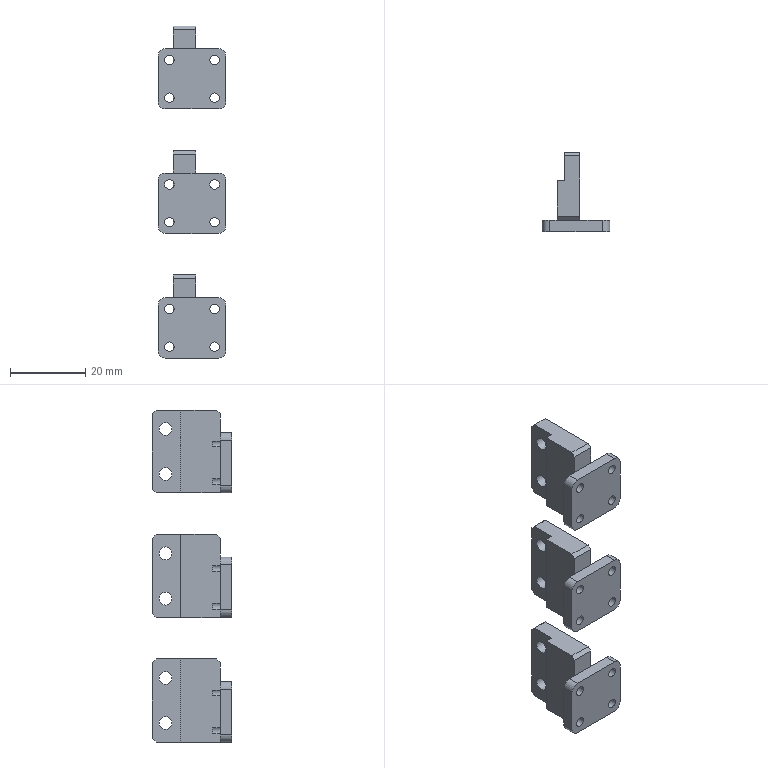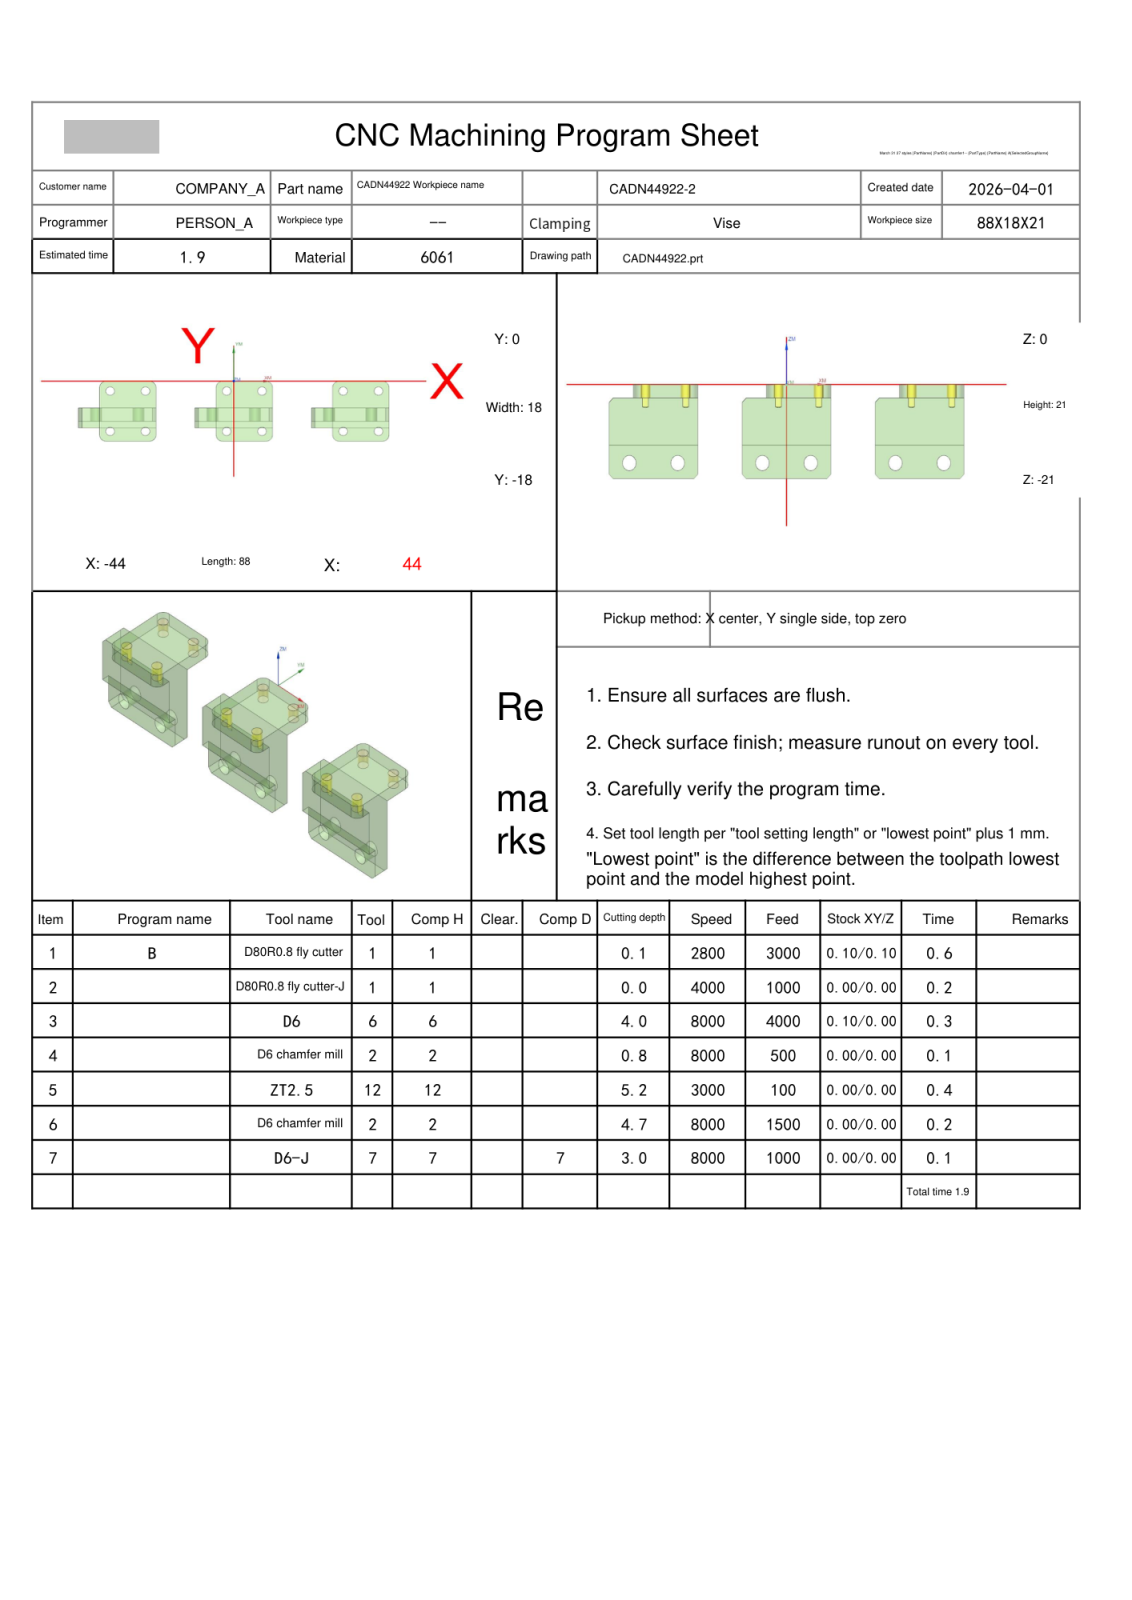NC program | NX | posted by the shop | part box 18 x 21 x 88 mm
Whole program:
%
O0001
(Machine time: 3.18 MIN)
(===Total Tool:5===)
(T1=D80R0.8 fly cutter D=80.  R=0.8  D-  H01 Z=0.    )
(T6=D6      D=6.   R=0.   D-  H06 Z=-4.   )
(T2=D6 chamfer mill   D=6.   R=0.   D-  H02 Z=-4.7  )
(T12=ZT2.5  D=2.5  DR_a=118 D-  H12 Z=-5.15 )
(T7=D6-J    D=6.   R=0.   D7  H07 Z=-3.   )
G80 G90 G17 G49 G40
G91 G28 Z0
M01
N1 T01 M06
(D80R0.8 fly cutter  D=80. R=0.8 H=01 ce=0.10 di=0.10)
G00 G90 G54 X96.097 Y-9. M03 S2800
G43 H01 Z20.
M08
Z5.014
G01 Z3.014 F3000.
X84.097
X-84.097
X-96.097
Z5.014
G00 X96.097
Z4.529
G01 Z2.529
X84.097
X-84.097
X-96.097
Z4.529
G00 X96.097
Z4.043
G01 Z2.043
X84.097
X-84.097
X-96.097
Z4.043
G00 X96.097
Z3.557
G01 Z1.557
X84.097
X-84.097
X-96.097
Z3.557
G00 Z20.
X96.097
Z3.071
G01 Z1.071
X84.097
X-84.097
X-96.097
Z3.071
G00 Z20.
X96.097
Z2.586
G01 Z.586
X84.097
X-84.097
X-96.097
Z2.586
G00 Z20.
X96.097
Z2.1
G01 Z.1
X84.097
X-84.097
X-96.097
Z2.1
G00 Z20.
G91 G28 Z0.0
M05
M09
G91 G28 Z0.0
M01
N2 T01 M06
(D80R0.8 fly cutter-J  D=80. R=0.8 H=01 ce=0.00 di=0.00)
G00 G90 G54 X95.999 Y-9. M03 S4000
G43 H01 Z20.
M08
Z2.
G01 Z0.0 F1000.
X83.999
X-83.999
X-95.999
Z2.
G00 Z20.
G91 G28 Z0.0
M05
M09
G91 G28 Z0.0
M01
N3 T06 M06
(D6  D=6. R=0. H=06 ce=0.10 di=0.10)
G00 G90 G54 X-45.6 Y-2. M03 S8000
G43 H06 Z13.8
M08
Z1.017
G01 Z-.483 F3000.
Y-5.06
Y-16.
G03 X-45.589 Y-16.462 I9.6 J0.0
X-45.097 Y-17.023 I.599 J.029
G01 X-41.71 Y-17.641
X-41.602 Y-17.651
G03 X-41.002 Y-17.051 I0.0 J.6
G01 X-41.013 Y-16.94
G02 X-41.1 Y-16. I5.013 J.94
G01 Y-5.06
Y-2.06
X-44.1 Y-2.
Z1.017
G00 X-45.6
Z.533
G01 Z-.967
Y-5.06
Y-16.
G03 X-45.589 Y-16.462 I9.6 J0.0
X-45.097 Y-17.023 I.599 J.029
G01 X-41.71 Y-17.641
X-41.602 Y-17.651
G03 X-41.002 Y-17.051 I0.0 J.6
G01 X-41.013 Y-16.94
G02 X-41.1 Y-16. I5.013 J.94
G01 Y-5.06
Y-2.06
X-44.1 Y-2.
Z.533
G00 X-45.6
Z.05
G01 Z-1.45
Y-5.06
Y-16.
G03 X-45.589 Y-16.462 I9.6 J0.0
X-45.097 Y-17.023 I.599 J.029
G01 X-41.71 Y-17.641
X-41.602 Y-17.651
G03 X-41.002 Y-17.051 I0.0 J.6
G01 X-41.013 Y-16.94
G02 X-41.1 Y-16. I5.013 J.94
G01 Y-5.06
Y-2.06
X-44.1 Y-2.
Z.05
G00 X-45.6
Z-.433
G01 Z-1.933
Y-5.06
Y-16.
G03 X-45.589 Y-16.462 I9.6 J0.0
X-45.097 Y-17.023 I.599 J.029
G01 X-41.71 Y-17.641
X-41.602 Y-17.651
G03 X-41.002 Y-17.051 I0.0 J.6
G01 X-41.013 Y-16.94
G02 X-41.1 Y-16. I5.013 J.94
G01 Y-5.06
Y-2.06
X-44.1 Y-2.
Z-.433
G00 X-45.6
Z-.917
G01 Z-2.417
Y-5.06
Y-16.
G03 X-45.589 Y-16.462 I9.6 J0.0
X-45.097 Y-17.023 I.599 J.029
G01 X-41.71 Y-17.641
X-41.602 Y-17.651
G03 X-41.002 Y-17.051 I0.0 J.6
G01 X-41.013 Y-16.94
G02 X-41.1 Y-16. I5.013 J.94
G01 Y-5.06
Y-2.06
X-44.1 Y-2.
Z-.917
G00 X-45.6
Z-1.4
G01 Z-2.9
Y-5.06
Y-16.
G03 X-45.589 Y-16.462 I9.6 J0.0
X-45.097 Y-17.023 I.599 J.029
G01 X-41.71 Y-17.641
X-41.602 Y-17.651
G03 X-41.002 Y-17.051 I0.0 J.6
G01 X-41.013 Y-16.94
G02 X-41.1 Y-16. I5.013 J.94
G01 Y-5.06
Y-2.06
X-44.1 Y-2.
Z-1.4
G00 Z13.8
X-12.6
Z1.017
G01 Z-.483
Y-5.06
Y-16.
G03 X-12.589 Y-16.462 I9.6 J0.0
X-12.097 Y-17.023 I.599 J.029
G01 X-8.71 Y-17.641
X-8.602 Y-17.651
G03 X-8.002 Y-17.051 I0.0 J.6
G01 X-8.013 Y-16.94
G02 X-8.1 Y-16. I5.013 J.94
G01 Y-5.06
Y-2.06
X-11.1 Y-2.
Z1.017
G00 X-12.6
Z.533
G01 Z-.967
Y-5.06
Y-16.
G03 X-12.589 Y-16.462 I9.6 J0.0
X-12.097 Y-17.023 I.599 J.029
G01 X-8.71 Y-17.641
X-8.602 Y-17.651
G03 X-8.002 Y-17.051 I0.0 J.6
G01 X-8.013 Y-16.94
G02 X-8.1 Y-16. I5.013 J.94
G01 Y-5.06
Y-2.06
X-11.1 Y-2.
Z.533
G00 X-12.6
Z.05
G01 Z-1.45
Y-5.06
Y-16.
G03 X-12.589 Y-16.462 I9.6 J0.0
X-12.097 Y-17.023 I.599 J.029
G01 X-8.71 Y-17.641
X-8.602 Y-17.651
G03 X-8.002 Y-17.051 I0.0 J.6
G01 X-8.013 Y-16.94
G02 X-8.1 Y-16. I5.013 J.94
G01 Y-5.06
Y-2.06
X-11.1 Y-2.
Z.05
G00 X-12.6
Z-.433
G01 Z-1.933
Y-5.06
Y-16.
G03 X-12.589 Y-16.462 I9.6 J0.0
X-12.097 Y-17.023 I.599 J.029
G01 X-8.71 Y-17.641
X-8.602 Y-17.651
G03 X-8.002 Y-17.051 I0.0 J.6
G01 X-8.013 Y-16.94
G02 X-8.1 Y-16. I5.013 J.94
G01 Y-5.06
Y-2.06
X-11.1 Y-2.
Z-.433
G00 X-12.6
Z-.917
G01 Z-2.417
Y-5.06
Y-16.
G03 X-12.589 Y-16.462 I9.6 J0.0
X-12.097 Y-17.023 I.599 J.029
G01 X-8.71 Y-17.641
X-8.602 Y-17.651
G03 X-8.002 Y-17.051 I0.0 J.6
G01 X-8.013 Y-16.94
G02 X-8.1 Y-16. I5.013 J.94
G01 Y-5.06
Y-2.06
X-11.1 Y-2.
Z-.917
G00 X-12.6
Z-1.4
G01 Z-2.9
Y-5.06
Y-16.
G03 X-12.589 Y-16.462 I9.6 J0.0
X-12.097 Y-17.023 I.599 J.029
G01 X-8.71 Y-17.641
X-8.602 Y-17.651
G03 X-8.002 Y-17.051 I0.0 J.6
G01 X-8.013 Y-16.94
G02 X-8.1 Y-16. I5.013 J.94
G01 Y-5.06
Y-2.06
X-11.1 Y-2.
Z-1.4
G00 Z13.8
X20.4
Z1.017
G01 Z-.483
Y-5.06
Y-16.
G03 X20.411 Y-16.462 I9.6 J0.0
X20.903 Y-17.023 I.599 J.029
G01 X24.29 Y-17.641
X24.398 Y-17.651
G03 X24.998 Y-17.051 I0.0 J.6
G01 X24.987 Y-16.94
G02 X24.9 Y-16. I5.013 J.94
G01 Y-5.06
Y-2.06
X21.9 Y-2.
Z1.017
G00 X20.4
Z.533
G01 Z-.967
Y-5.06
Y-16.
G03 X20.411 Y-16.462 I9.6 J0.0
X20.903 Y-17.023 I.599 J.029
G01 X24.29 Y-17.641
X24.398 Y-17.651
G03 X24.998 Y-17.051 I0.0 J.6
G01 X24.987 Y-16.94
G02 X24.9 Y-16. I5.013 J.94
G01 Y-5.06
Y-2.06
X21.9 Y-2.
Z.533
G00 X20.4
Z.05
G01 Z-1.45
Y-5.06
Y-16.
G03 X20.411 Y-16.462 I9.6 J0.0
X20.903 Y-17.023 I.599 J.029
G01 X24.29 Y-17.641
X24.398 Y-17.651
G03 X24.998 Y-17.051 I0.0 J.6
G01 X24.987 Y-16.94
G02 X24.9 Y-16. I5.013 J.94
G01 Y-5.06
Y-2.06
X21.9 Y-2.
Z.05
G00 X20.4
Z-.433
G01 Z-1.933
Y-5.06
Y-16.
G03 X20.411 Y-16.462 I9.6 J0.0
X20.903 Y-17.023 I.599 J.029
G01 X24.29 Y-17.641
X24.398 Y-17.651
G03 X24.998 Y-17.051 I0.0 J.6
G01 X24.987 Y-16.94
G02 X24.9 Y-16. I5.013 J.94
G01 Y-5.06
Y-2.06
X21.9 Y-2.
Z-.433
G00 X20.4
Z-.917
G01 Z-2.417
Y-5.06
Y-16.
G03 X20.411 Y-16.462 I9.6 J0.0
X20.903 Y-17.023 I.599 J.029
G01 X24.29 Y-17.641
X24.398 Y-17.651
G03 X24.998 Y-17.051 I0.0 J.6
G01 X24.987 Y-16.94
G02 X24.9 Y-16. I5.013 J.94
G01 Y-5.06
Y-2.06
X21.9 Y-2.
Z-.917
G00 X20.4
Z-1.4
G01 Z-2.9
Y-5.06
Y-16.
G03 X20.411 Y-16.462 I9.6 J0.0
X20.903 Y-17.023 I.599 J.029
G01 X24.29 Y-17.641
X24.398 Y-17.651
G03 X24.998 Y-17.051 I0.0 J.6
G01 X24.987 Y-16.94
G02 X24.9 Y-16. I5.013 J.94
G01 Y-5.06
Y-2.06
X21.9 Y-2.
Z-1.4
G00 Z13.8
G00 G90 X-46.185 Y-20.358 M03 S7000
Z13.8
Z-2.641
G01 Z-3.141 F4000.
X-46.239 Y-15.071
X-46.241 Y-14.87
Y-7.13
X-46.239 Y-6.928
X-46.312 Z-3.212
X-46.381 Z-3.283
X-46.383 Y-7.13
Y-14.87
X-46.381 Y-15.071
X-46.454 Z-3.354
X-46.522 Z-3.424
X-46.524 Y-14.87
Y-7.13
X-46.522 Y-6.928
X-46.595 Z-3.495
X-46.664 Z-3.566
X-46.666 Y-7.13
Y-14.87
X-46.664 Y-15.071
X-46.72 Z-3.62
X-46.772 Z-3.674
X-46.774 Y-14.87
Y-7.13
X-46.772 Y-6.928
X-46.829 Z-3.729
X-46.881 Z-3.783
X-46.883 Y-7.13
Y-14.87
X-46.881 Y-15.071
X-46.937 Z-3.837
X-46.989 Z-3.891
X-46.991 Y-14.87
Y-7.13
X-46.989 Y-6.928
X-47.046 Z-3.946
X-47.098 Z-4.
X-47.1 Y-7.13
Y-14.87
X-47.098 Y-15.071
G00 Z13.8
X-13.185 Y-20.357
Z-2.641
G01 Z-3.141
X-13.239 Y-15.071
X-13.241 Y-14.87
Y-7.13
X-13.239 Y-6.928
X-13.312 Z-3.212
X-13.381 Z-3.283
X-13.383 Y-7.13
Y-14.87
X-13.381 Y-15.071
X-13.454 Z-3.354
X-13.522 Z-3.424
X-13.524 Y-14.87
Y-7.13
X-13.522 Y-6.928
X-13.595 Z-3.495
X-13.664 Z-3.566
X-13.666 Y-7.13
Y-14.87
X-13.664 Y-15.071
X-13.72 Z-3.62
X-13.772 Z-3.674
X-13.774 Y-14.87
Y-7.13
X-13.772 Y-6.928
X-13.829 Z-3.729
X-13.881 Z-3.783
X-13.883 Y-7.13
Y-14.87
X-13.881 Y-15.071
X-13.937 Z-3.837
X-13.989 Z-3.891
X-13.991 Y-14.87
Y-7.13
X-13.989 Y-6.928
X-14.046 Z-3.946
X-14.098 Z-4.
X-14.1 Y-7.13
Y-14.87
X-14.098 Y-15.071
G00 Z13.8
X19.815 Y-20.357
Z-2.641
G01 Z-3.141
X19.761 Y-15.071
X19.759 Y-14.87
Y-7.13
X19.761 Y-6.928
X19.688 Z-3.212
X19.619 Z-3.283
X19.617 Y-7.13
Y-14.87
X19.619 Y-15.071
X19.546 Z-3.354
X19.478 Z-3.424
X19.476 Y-14.87
Y-7.13
X19.478 Y-6.928
X19.405 Z-3.495
X19.336 Z-3.566
X19.334 Y-7.13
Y-14.87
X19.336 Y-15.071
X19.28 Z-3.62
X19.228 Z-3.674
X19.226 Y-14.87
Y-7.13
X19.228 Y-6.928
X19.171 Z-3.729
X19.119 Z-3.783
X19.117 Y-7.13
Y-14.87
X19.119 Y-15.071
X19.063 Z-3.837
X19.011 Z-3.891
X19.009 Y-14.87
Y-7.13
X19.011 Y-6.928
X18.954 Z-3.946
X18.902 Z-4.
X18.9 Y-7.13
Y-14.87
X18.902 Y-15.071
G00 Z13.8
G91 G28 Z0.0
M05
M09
G91 G28 Z0.0
M01
N4 T02 M06
(D6 chamfer mill  D=6. R=0. H=02 ce=0.00 di=0.00)
G00 G90 G54 X31. Y-3. M03 S8000
G43 H02 Z20.
M08
G98 G81 X31. Y-3. Z-.8 R1. F500.
X41.
Y-15.
X31.
X8.
Y-3.
X-2.
Y-15.
X-25.
X-35.
Y-3.
X-25.
G80
G00 Z20.
G91 G28 Z0.0
M05
M09
G91 G28 Z0.0
M01
N5 T12 M06
(ZT2.5 D=2.5 DR_a=118 H=12)
G00 G90 G54 X41. Y-15. M03 S3000
G43 H12 Z20.
M08
G98 G83 X41. Y-15. Z-5.15 R1. F100. Q2.
X31.
X8.
X-2.
X-25.
X-35.
G80
G00 Z20.
G91 G28 Z0.0
M05
M09
G91 G28 Z0.0
M01
N6 T02 M06
(D6 chamfer mill  D=6. R=0. H=02 ce=0.00 di=0.00)
G00 G90 G54 X31. Y-3. M03 S8000
G43 H02 Z20.
M08
G98 G81 X31. Y-3. Z-1.75 R3. F500.
X41.
Y-15.
X31.
X8.
Y-3.
X-2.
Y-15.
X-25.
X-35.
Y-3.
X-25.
G80
G00 Z20.
G00 G90 X21.292 Y-16.9 M03 S6500
Z20.
Z-3.2
G01 Z-4.7 F1500.
X21.301 Y-16.832
X21.3 Y-16.763
Y-5.237
X21.301 Y-5.168
X21.292 Y-5.1
Z-3.2
G00 Z20.
X-11.708 Y-16.9
Z-3.2
G01 Z-4.7
X-11.699 Y-16.832
X-11.7 Y-16.763
Y-5.237
X-11.699 Y-5.168
X-11.708 Y-5.1
Z-3.2
G00 Z20.
X-44.708 Y-16.9
Z-3.2
G01 Z-4.7
X-44.699 Y-16.832
X-44.7 Y-16.763
Y-5.237
X-44.699 Y-5.168
X-44.708 Y-5.1
Z-3.2
G00 Z20.
G91 G28 Z0.0
M05
M09
G91 G28 Z0.0
M01
N7 T07 M06
(D6-J  D=6. R=0. H=07 ce=0.00 di=0.00)
G00 G90 G54 X23.991 Y-18.202 M03 S8000
G43 H07 Z13.8
M08
Z-2.
G01 Z-3. F1000.
G41 D07
X24.18 Y-18.138
G03 X25. Y-17. I-.38 J1.138
G01 Y-5.
G03 X23.8 Y-3.8 I-1.2 J0.0
G01 G40 X23.6
Z-2.
G00 Z13.8
X-9.009 Y-18.202
Z-2.
G01 Z-3.
G41 D07
X-8.82 Y-18.138
G03 X-8. Y-17. I-.38 J1.138
G01 Y-5.
G03 X-9.2 Y-3.8 I-1.2 J0.0
G01 G40 X-9.4
Z-2.
G00 Z13.8
X-42.009 Y-18.202
Z-2.
G01 Z-3.
G41 D07
X-41.82 Y-18.138
G03 X-41. Y-17. I-.38 J1.138
G01 Y-5.
G03 X-42.2 Y-3.8 I-1.2 J0.0
G01 G40 X-42.4
Z-2.
G00 Z13.8
M05
M09
G91 G28 Z0.0
G91 G28 Y0.0
M30
%